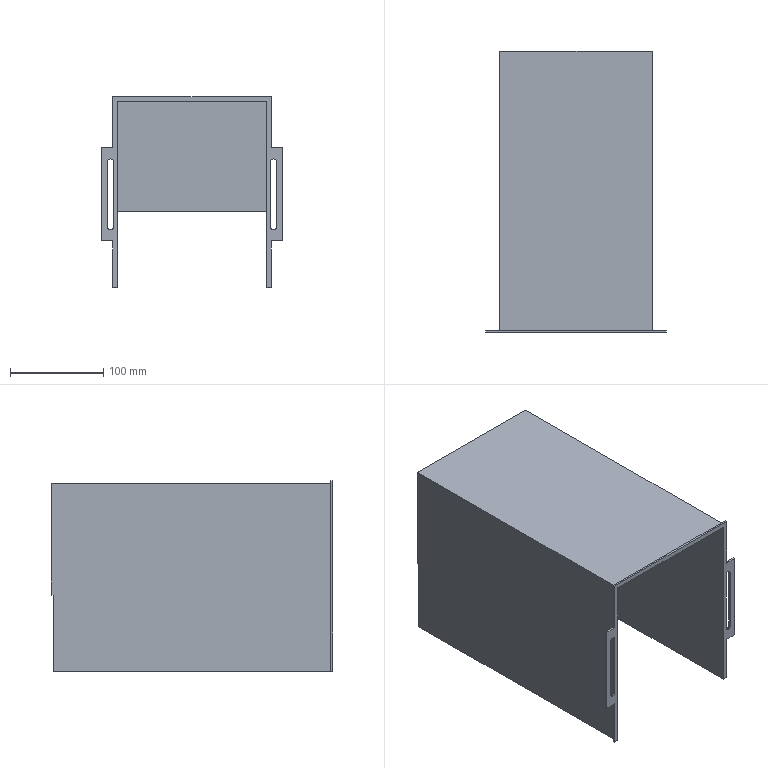Part | SolidWorks | features ICE 4, Extrusion 1 | 1 solid | 36 faces | box 194 x 302 x 205 mm | volume 384147 mm3 | plane 30 | cylinder 6 | commonest cylinder face diameters 6.2 x6
STEP:
#1=CARTESIAN_POINT('',(-4.4,2.,-135.));
#2=VERTEX_POINT('',#1);
#3=CARTESIAN_POINT('',(-7.5,2.,-138.1));
#4=VERTEX_POINT('',#3);
#5=CARTESIAN_POINT('',(-7.5,2.,-135.));
#6=DIRECTION('',(0.,1.,0.));
#7=DIRECTION('',(0.,0.,1.));
#8=AXIS2_PLACEMENT_3D('',#5,#6,#7);
#9=CIRCLE('',#8,3.1);
#10=EDGE_CURVE('',#2,#4,#9,.T.);
#11=ORIENTED_EDGE('',*,*,#10,.T.);
#12=CARTESIAN_POINT('',(-7.5,0.,-138.1));
#13=VERTEX_POINT('',#12);
#14=CARTESIAN_POINT('',(-7.5,300.,-138.1));
#15=DIRECTION('',(0.,-1.,0.));
#16=VECTOR('',#15,1000.);
#17=LINE('',#14,#16);
#18=EDGE_CURVE('',#4,#13,#17,.T.);
#19=ORIENTED_EDGE('',*,*,#18,.T.);
#20=CARTESIAN_POINT('',(-4.4,0.,-135.));
#21=VERTEX_POINT('',#20);
#22=CARTESIAN_POINT('',(-7.5,0.,-135.));
#23=DIRECTION('',(0.,-1.,0.));
#24=DIRECTION('',(0.,0.,-1.));
#25=AXIS2_PLACEMENT_3D('',#22,#23,#24);
#26=CIRCLE('',#25,3.1);
#27=EDGE_CURVE('',#13,#21,#26,.T.);
#28=ORIENTED_EDGE('',*,*,#27,.T.);
#29=CARTESIAN_POINT('',(-4.4,300.,-135.));
#30=DIRECTION('',(0.,-1.,0.));
#31=VECTOR('',#30,1000.);
#32=LINE('',#29,#31);
#33=EDGE_CURVE('',#2,#21,#32,.T.);
#34=ORIENTED_EDGE('',*,*,#33,.F.);
#35=EDGE_LOOP('',(#11,#19,#28,#34));
#36=FACE_OUTER_BOUND('',#35,.T.);
#37=CARTESIAN_POINT('',(-7.5,300.,-135.));
#38=DIRECTION('',(0.,-1.,0.));
#39=DIRECTION('',(0.,0.,-1.));
#40=AXIS2_PLACEMENT_3D('',#37,#38,#39);
#41=CYLINDRICAL_SURFACE('',#40,3.1);
#42=ADVANCED_FACE('',(#36),#41,.F.);
#43=CARTESIAN_POINT('',(167.5,2.,-138.1));
#44=VERTEX_POINT('',#43);
#45=CARTESIAN_POINT('',(170.6,2.,-135.));
#46=VERTEX_POINT('',#45);
#47=CARTESIAN_POINT('',(167.5,2.,-135.));
#48=DIRECTION('',(0.,-1.,0.));
#49=DIRECTION('',(0.,0.,-1.));
#50=AXIS2_PLACEMENT_3D('',#47,#48,#49);
#51=CIRCLE('',#50,3.1);
#52=EDGE_CURVE('',#44,#46,#51,.T.);
#53=ORIENTED_EDGE('',*,*,#52,.F.);
#54=CARTESIAN_POINT('',(167.5,0.,-138.1));
#55=VERTEX_POINT('',#54);
#56=CARTESIAN_POINT('',(167.5,300.,-138.1));
#57=DIRECTION('',(0.,-1.,0.));
#58=VECTOR('',#57,1000.);
#59=LINE('',#56,#58);
#60=EDGE_CURVE('',#44,#55,#59,.T.);
#61=ORIENTED_EDGE('',*,*,#60,.T.);
#62=CARTESIAN_POINT('',(170.6,0.,-135.));
#63=VERTEX_POINT('',#62);
#64=CARTESIAN_POINT('',(167.5,0.,-135.));
#65=DIRECTION('',(0.,-1.,0.));
#66=DIRECTION('',(0.,0.,-1.));
#67=AXIS2_PLACEMENT_3D('',#64,#65,#66);
#68=CIRCLE('',#67,3.1);
#69=EDGE_CURVE('',#55,#63,#68,.T.);
#70=ORIENTED_EDGE('',*,*,#69,.T.);
#71=CARTESIAN_POINT('',(170.6,300.,-135.));
#72=DIRECTION('',(0.,-1.,0.));
#73=VECTOR('',#72,1000.);
#74=LINE('',#71,#73);
#75=EDGE_CURVE('',#46,#63,#74,.T.);
#76=ORIENTED_EDGE('',*,*,#75,.F.);
#77=EDGE_LOOP('',(#53,#61,#70,#76));
#78=FACE_OUTER_BOUND('',#77,.T.);
#79=CARTESIAN_POINT('',(167.5,300.,-135.));
#80=DIRECTION('',(0.,-1.,0.));
#81=DIRECTION('',(0.,0.,-1.));
#82=AXIS2_PLACEMENT_3D('',#79,#80,#81);
#83=CYLINDRICAL_SURFACE('',#82,3.1);
#84=ADVANCED_FACE('',(#78),#83,.F.);
#85=CARTESIAN_POINT('',(162.,2.,2.));
#86=VERTEX_POINT('',#85);
#87=CARTESIAN_POINT('',(162.,2.,-200.));
#88=VERTEX_POINT('',#87);
#89=CARTESIAN_POINT('',(162.,2.,-50.));
#90=DIRECTION('',(0.,0.,-1.));
#91=VECTOR('',#90,1000.);
#92=LINE('',#89,#91);
#93=EDGE_CURVE('',#86,#88,#92,.T.);
#94=ORIENTED_EDGE('',*,*,#93,.T.);
#95=CARTESIAN_POINT('',(162.,300.,-200.));
#96=VERTEX_POINT('',#95);
#97=CARTESIAN_POINT('',(162.,300.,-200.));
#98=DIRECTION('',(0.,-1.,0.));
#99=VECTOR('',#98,1000.);
#100=LINE('',#97,#99);
#101=EDGE_CURVE('',#96,#88,#100,.T.);
#102=ORIENTED_EDGE('',*,*,#101,.F.);
#103=CARTESIAN_POINT('',(162.,300.,-118.));
#104=VERTEX_POINT('',#103);
#105=CARTESIAN_POINT('',(162.,300.,2.));
#106=DIRECTION('',(0.,0.,-1.));
#107=VECTOR('',#106,1000.);
#108=LINE('',#105,#107);
#109=EDGE_CURVE('',#104,#96,#108,.T.);
#110=ORIENTED_EDGE('',*,*,#109,.F.);
#111=CARTESIAN_POINT('',(162.,302.,-118.));
#112=VERTEX_POINT('',#111);
#113=CARTESIAN_POINT('',(162.,302.,-118.));
#114=DIRECTION('',(0.,-1.,0.));
#115=VECTOR('',#114,1000.);
#116=LINE('',#113,#115);
#117=EDGE_CURVE('',#112,#104,#116,.T.);
#118=ORIENTED_EDGE('',*,*,#117,.F.);
#119=CARTESIAN_POINT('',(162.,302.,2.));
#120=VERTEX_POINT('',#119);
#121=CARTESIAN_POINT('',(162.,302.,2.));
#122=DIRECTION('',(0.,0.,-1.));
#123=VECTOR('',#122,1000.);
#124=LINE('',#121,#123);
#125=EDGE_CURVE('',#120,#112,#124,.T.);
#126=ORIENTED_EDGE('',*,*,#125,.F.);
#127=CARTESIAN_POINT('',(162.,300.,2.));
#128=DIRECTION('',(0.,-1.,0.));
#129=VECTOR('',#128,1000.);
#130=LINE('',#127,#129);
#131=EDGE_CURVE('',#120,#86,#130,.T.);
#132=ORIENTED_EDGE('',*,*,#131,.T.);
#133=EDGE_LOOP('',(#94,#102,#110,#118,#126,#132));
#134=FACE_OUTER_BOUND('',#133,.T.);
#135=CARTESIAN_POINT('',(162.,300.,2.));
#136=DIRECTION('',(-1.,0.,0.));
#137=DIRECTION('',(0.,0.,1.));
#138=AXIS2_PLACEMENT_3D('',#135,#136,#137);
#139=PLANE('',#138);
#140=ADVANCED_FACE('',(#134),#139,.F.);
#141=CARTESIAN_POINT('',(-2.,2.,-200.));
#142=VERTEX_POINT('',#141);
#143=CARTESIAN_POINT('',(-2.,2.,2.));
#144=VERTEX_POINT('',#143);
#145=CARTESIAN_POINT('',(-2.,2.,-50.));
#146=DIRECTION('',(0.,0.,1.));
#147=VECTOR('',#146,1000.);
#148=LINE('',#145,#147);
#149=EDGE_CURVE('',#142,#144,#148,.T.);
#150=ORIENTED_EDGE('',*,*,#149,.T.);
#151=CARTESIAN_POINT('',(-2.,302.,2.));
#152=VERTEX_POINT('',#151);
#153=CARTESIAN_POINT('',(-2.,300.,2.));
#154=DIRECTION('',(0.,-1.,0.));
#155=VECTOR('',#154,1000.);
#156=LINE('',#153,#155);
#157=EDGE_CURVE('',#152,#144,#156,.T.);
#158=ORIENTED_EDGE('',*,*,#157,.F.);
#159=CARTESIAN_POINT('',(-2.,302.,-118.));
#160=VERTEX_POINT('',#159);
#161=CARTESIAN_POINT('',(-2.,302.,2.));
#162=DIRECTION('',(0.,0.,1.));
#163=VECTOR('',#162,1000.);
#164=LINE('',#161,#163);
#165=EDGE_CURVE('',#160,#152,#164,.T.);
#166=ORIENTED_EDGE('',*,*,#165,.F.);
#167=CARTESIAN_POINT('',(-2.,300.,-118.));
#168=VERTEX_POINT('',#167);
#169=CARTESIAN_POINT('',(-2.,302.,-118.));
#170=DIRECTION('',(0.,-1.,0.));
#171=VECTOR('',#170,1000.);
#172=LINE('',#169,#171);
#173=EDGE_CURVE('',#160,#168,#172,.T.);
#174=ORIENTED_EDGE('',*,*,#173,.T.);
#175=CARTESIAN_POINT('',(-2.,300.,-200.));
#176=VERTEX_POINT('',#175);
#177=CARTESIAN_POINT('',(-2.,300.,2.));
#178=DIRECTION('',(0.,0.,1.));
#179=VECTOR('',#178,1000.);
#180=LINE('',#177,#179);
#181=EDGE_CURVE('',#176,#168,#180,.T.);
#182=ORIENTED_EDGE('',*,*,#181,.F.);
#183=CARTESIAN_POINT('',(-2.,300.,-200.));
#184=DIRECTION('',(0.,-1.,0.));
#185=VECTOR('',#184,1000.);
#186=LINE('',#183,#185);
#187=EDGE_CURVE('',#176,#142,#186,.T.);
#188=ORIENTED_EDGE('',*,*,#187,.T.);
#189=EDGE_LOOP('',(#150,#158,#166,#174,#182,#188));
#190=FACE_OUTER_BOUND('',#189,.T.);
#191=CARTESIAN_POINT('',(-2.,300.,2.));
#192=DIRECTION('',(1.,0.,0.));
#193=DIRECTION('',(0.,0.,-1.));
#194=AXIS2_PLACEMENT_3D('',#191,#192,#193);
#195=PLANE('',#194);
#196=ADVANCED_FACE('',(#190),#195,.F.);
#197=CARTESIAN_POINT('',(-2.,2.,2.));
#198=DIRECTION('',(1.,0.,0.));
#199=VECTOR('',#198,1000.);
#200=LINE('',#197,#199);
#201=EDGE_CURVE('',#144,#86,#200,.T.);
#202=ORIENTED_EDGE('',*,*,#201,.T.);
#203=ORIENTED_EDGE('',*,*,#131,.F.);
#204=CARTESIAN_POINT('',(-2.,302.,2.));
#205=DIRECTION('',(1.,0.,0.));
#206=VECTOR('',#205,1000.);
#207=LINE('',#204,#206);
#208=EDGE_CURVE('',#152,#120,#207,.T.);
#209=ORIENTED_EDGE('',*,*,#208,.F.);
#210=ORIENTED_EDGE('',*,*,#157,.T.);
#211=EDGE_LOOP('',(#202,#203,#209,#210));
#212=FACE_OUTER_BOUND('',#211,.T.);
#213=CARTESIAN_POINT('',(-2.,300.,2.));
#214=DIRECTION('',(0.,0.,-1.));
#215=DIRECTION('',(-1.,0.,0.));
#216=AXIS2_PLACEMENT_3D('',#213,#214,#215);
#217=PLANE('',#216);
#218=ADVANCED_FACE('',(#212),#217,.F.);
#219=CARTESIAN_POINT('',(160.,300.,-118.));
#220=VERTEX_POINT('',#219);
#221=CARTESIAN_POINT('',(-2.,300.,-118.));
#222=DIRECTION('',(-1.,0.,0.));
#223=VECTOR('',#222,1000.);
#224=LINE('',#221,#223);
#225=EDGE_CURVE('',#104,#220,#224,.T.);
#226=ORIENTED_EDGE('',*,*,#225,.F.);
#227=ORIENTED_EDGE('',*,*,#109,.T.);
#228=CARTESIAN_POINT('',(160.,300.,-200.));
#229=VERTEX_POINT('',#228);
#230=CARTESIAN_POINT('',(160.,300.,-200.));
#231=DIRECTION('',(-1.,0.,0.));
#232=VECTOR('',#231,1000.);
#233=LINE('',#230,#232);
#234=EDGE_CURVE('',#96,#229,#233,.T.);
#235=ORIENTED_EDGE('',*,*,#234,.T.);
#236=CARTESIAN_POINT('',(160.,300.,0.));
#237=DIRECTION('',(0.,0.,1.));
#238=VECTOR('',#237,1000.);
#239=LINE('',#236,#238);
#240=EDGE_CURVE('',#229,#220,#239,.T.);
#241=ORIENTED_EDGE('',*,*,#240,.T.);
#242=EDGE_LOOP('',(#226,#227,#235,#241));
#243=FACE_OUTER_BOUND('',#242,.T.);
#244=CARTESIAN_POINT('',(0.,300.,0.));
#245=DIRECTION('',(0.,1.,0.));
#246=DIRECTION('',(0.,0.,1.));
#247=AXIS2_PLACEMENT_3D('',#244,#245,#246);
#248=PLANE('',#247);
#249=ADVANCED_FACE('',(#243),#248,.T.);
#250=CARTESIAN_POINT('',(160.,0.,0.));
#251=VERTEX_POINT('',#250);
#252=CARTESIAN_POINT('',(0.,0.,0.));
#253=VERTEX_POINT('',#252);
#254=CARTESIAN_POINT('',(0.,0.,0.));
#255=DIRECTION('',(-1.,0.,0.));
#256=VECTOR('',#255,1000.);
#257=LINE('',#254,#256);
#258=EDGE_CURVE('',#251,#253,#257,.T.);
#259=ORIENTED_EDGE('',*,*,#258,.T.);
#260=CARTESIAN_POINT('',(0.,300.,0.));
#261=VERTEX_POINT('',#260);
#262=CARTESIAN_POINT('',(0.,300.,0.));
#263=DIRECTION('',(0.,-1.,0.));
#264=VECTOR('',#263,1000.);
#265=LINE('',#262,#264);
#266=EDGE_CURVE('',#261,#253,#265,.T.);
#267=ORIENTED_EDGE('',*,*,#266,.F.);
#268=CARTESIAN_POINT('',(160.,300.,0.));
#269=VERTEX_POINT('',#268);
#270=CARTESIAN_POINT('',(0.,300.,0.));
#271=DIRECTION('',(-1.,0.,0.));
#272=VECTOR('',#271,1000.);
#273=LINE('',#270,#272);
#274=EDGE_CURVE('',#269,#261,#273,.T.);
#275=ORIENTED_EDGE('',*,*,#274,.F.);
#276=CARTESIAN_POINT('',(160.,300.,0.));
#277=DIRECTION('',(0.,-1.,0.));
#278=VECTOR('',#277,1000.);
#279=LINE('',#276,#278);
#280=EDGE_CURVE('',#269,#251,#279,.T.);
#281=ORIENTED_EDGE('',*,*,#280,.T.);
#282=EDGE_LOOP('',(#259,#267,#275,#281));
#283=FACE_OUTER_BOUND('',#282,.T.);
#284=CARTESIAN_POINT('',(0.,300.,0.));
#285=DIRECTION('',(0.,0.,1.));
#286=DIRECTION('',(1.,0.,0.));
#287=AXIS2_PLACEMENT_3D('',#284,#285,#286);
#288=PLANE('',#287);
#289=ADVANCED_FACE('',(#283),#288,.F.);
#290=CARTESIAN_POINT('',(0.,0.,-200.));
#291=VERTEX_POINT('',#290);
#292=CARTESIAN_POINT('',(0.,0.,0.));
#293=DIRECTION('',(0.,0.,-1.));
#294=VECTOR('',#293,1000.);
#295=LINE('',#292,#294);
#296=EDGE_CURVE('',#253,#291,#295,.T.);
#297=ORIENTED_EDGE('',*,*,#296,.T.);
#298=CARTESIAN_POINT('',(0.,300.,-200.));
#299=VERTEX_POINT('',#298);
#300=CARTESIAN_POINT('',(0.,300.,-200.));
#301=DIRECTION('',(0.,-1.,0.));
#302=VECTOR('',#301,1000.);
#303=LINE('',#300,#302);
#304=EDGE_CURVE('',#299,#291,#303,.T.);
#305=ORIENTED_EDGE('',*,*,#304,.F.);
#306=CARTESIAN_POINT('',(0.,300.,-118.));
#307=VERTEX_POINT('',#306);
#308=CARTESIAN_POINT('',(0.,300.,0.));
#309=DIRECTION('',(0.,0.,-1.));
#310=VECTOR('',#309,1000.);
#311=LINE('',#308,#310);
#312=EDGE_CURVE('',#307,#299,#311,.T.);
#313=ORIENTED_EDGE('',*,*,#312,.F.);
#314=CARTESIAN_POINT('',(0.,300.,0.));
#315=DIRECTION('',(0.,0.,-1.));
#316=VECTOR('',#315,1000.);
#317=LINE('',#314,#316);
#318=EDGE_CURVE('',#261,#307,#317,.T.);
#319=ORIENTED_EDGE('',*,*,#318,.F.);
#320=ORIENTED_EDGE('',*,*,#266,.T.);
#321=EDGE_LOOP('',(#297,#305,#313,#319,#320));
#322=FACE_OUTER_BOUND('',#321,.T.);
#323=CARTESIAN_POINT('',(0.,300.,0.));
#324=DIRECTION('',(-1.,0.,0.));
#325=DIRECTION('',(0.,0.,1.));
#326=AXIS2_PLACEMENT_3D('',#323,#324,#325);
#327=PLANE('',#326);
#328=ADVANCED_FACE('',(#322),#327,.F.);
#329=CARTESIAN_POINT('',(-5.,0.,-200.));
#330=VERTEX_POINT('',#329);
#331=CARTESIAN_POINT('',(-2.,0.,-200.));
#332=DIRECTION('',(-1.,0.,0.));
#333=VECTOR('',#332,1000.);
#334=LINE('',#331,#333);
#335=EDGE_CURVE('',#291,#330,#334,.T.);
#336=ORIENTED_EDGE('',*,*,#335,.T.);
#337=CARTESIAN_POINT('',(-5.,2.,-200.));
#338=VERTEX_POINT('',#337);
#339=CARTESIAN_POINT('',(-5.,2.,-200.));
#340=DIRECTION('',(0.,-1.,0.));
#341=VECTOR('',#340,1000.);
#342=LINE('',#339,#341);
#343=EDGE_CURVE('',#338,#330,#342,.T.);
#344=ORIENTED_EDGE('',*,*,#343,.F.);
#345=CARTESIAN_POINT('',(-5.,2.,-200.));
#346=DIRECTION('',(1.,0.,0.));
#347=VECTOR('',#346,1000.);
#348=LINE('',#345,#347);
#349=EDGE_CURVE('',#338,#142,#348,.T.);
#350=ORIENTED_EDGE('',*,*,#349,.T.);
#351=ORIENTED_EDGE('',*,*,#187,.F.);
#352=CARTESIAN_POINT('',(-2.,300.,-200.));
#353=DIRECTION('',(-1.,0.,0.));
#354=VECTOR('',#353,1000.);
#355=LINE('',#352,#354);
#356=EDGE_CURVE('',#299,#176,#355,.T.);
#357=ORIENTED_EDGE('',*,*,#356,.F.);
#358=ORIENTED_EDGE('',*,*,#304,.T.);
#359=EDGE_LOOP('',(#336,#344,#350,#351,#357,#358));
#360=FACE_OUTER_BOUND('',#359,.T.);
#361=CARTESIAN_POINT('',(-2.,300.,-200.));
#362=DIRECTION('',(0.,0.,1.));
#363=DIRECTION('',(1.,0.,0.));
#364=AXIS2_PLACEMENT_3D('',#361,#362,#363);
#365=PLANE('',#364);
#366=ADVANCED_FACE('',(#360),#365,.F.);
#367=CARTESIAN_POINT('',(165.,0.,-200.));
#368=VERTEX_POINT('',#367);
#369=CARTESIAN_POINT('',(160.,0.,-200.));
#370=VERTEX_POINT('',#369);
#371=CARTESIAN_POINT('',(160.,0.,-200.));
#372=DIRECTION('',(-1.,0.,0.));
#373=VECTOR('',#372,1000.);
#374=LINE('',#371,#373);
#375=EDGE_CURVE('',#368,#370,#374,.T.);
#376=ORIENTED_EDGE('',*,*,#375,.T.);
#377=CARTESIAN_POINT('',(160.,300.,-200.));
#378=DIRECTION('',(0.,-1.,0.));
#379=VECTOR('',#378,1000.);
#380=LINE('',#377,#379);
#381=EDGE_CURVE('',#229,#370,#380,.T.);
#382=ORIENTED_EDGE('',*,*,#381,.F.);
#383=ORIENTED_EDGE('',*,*,#234,.F.);
#384=ORIENTED_EDGE('',*,*,#101,.T.);
#385=CARTESIAN_POINT('',(165.,2.,-200.));
#386=VERTEX_POINT('',#385);
#387=CARTESIAN_POINT('',(162.,2.,-200.));
#388=DIRECTION('',(1.,0.,0.));
#389=VECTOR('',#388,1000.);
#390=LINE('',#387,#389);
#391=EDGE_CURVE('',#88,#386,#390,.T.);
#392=ORIENTED_EDGE('',*,*,#391,.T.);
#393=CARTESIAN_POINT('',(165.,2.,-200.));
#394=DIRECTION('',(0.,-1.,0.));
#395=VECTOR('',#394,1000.);
#396=LINE('',#393,#395);
#397=EDGE_CURVE('',#386,#368,#396,.T.);
#398=ORIENTED_EDGE('',*,*,#397,.T.);
#399=EDGE_LOOP('',(#376,#382,#383,#384,#392,#398));
#400=FACE_OUTER_BOUND('',#399,.T.);
#401=CARTESIAN_POINT('',(160.,300.,-200.));
#402=DIRECTION('',(0.,0.,1.));
#403=DIRECTION('',(1.,0.,0.));
#404=AXIS2_PLACEMENT_3D('',#401,#402,#403);
#405=PLANE('',#404);
#406=ADVANCED_FACE('',(#400),#405,.F.);
#407=CARTESIAN_POINT('',(160.,0.,0.));
#408=DIRECTION('',(0.,0.,1.));
#409=VECTOR('',#408,1000.);
#410=LINE('',#407,#409);
#411=EDGE_CURVE('',#370,#251,#410,.T.);
#412=ORIENTED_EDGE('',*,*,#411,.T.);
#413=ORIENTED_EDGE('',*,*,#280,.F.);
#414=CARTESIAN_POINT('',(160.,300.,0.));
#415=DIRECTION('',(0.,0.,1.));
#416=VECTOR('',#415,1000.);
#417=LINE('',#414,#416);
#418=EDGE_CURVE('',#220,#269,#417,.T.);
#419=ORIENTED_EDGE('',*,*,#418,.F.);
#420=ORIENTED_EDGE('',*,*,#240,.F.);
#421=ORIENTED_EDGE('',*,*,#381,.T.);
#422=EDGE_LOOP('',(#412,#413,#419,#420,#421));
#423=FACE_OUTER_BOUND('',#422,.T.);
#424=CARTESIAN_POINT('',(160.,300.,0.));
#425=DIRECTION('',(1.,0.,0.));
#426=DIRECTION('',(0.,0.,-1.));
#427=AXIS2_PLACEMENT_3D('',#424,#425,#426);
#428=PLANE('',#427);
#429=ADVANCED_FACE('',(#423),#428,.F.);
#430=CARTESIAN_POINT('',(-2.,300.,-118.));
#431=DIRECTION('',(-1.,0.,0.));
#432=VECTOR('',#431,1000.);
#433=LINE('',#430,#432);
#434=EDGE_CURVE('',#307,#168,#433,.T.);
#435=ORIENTED_EDGE('',*,*,#434,.F.);
#436=ORIENTED_EDGE('',*,*,#312,.T.);
#437=ORIENTED_EDGE('',*,*,#356,.T.);
#438=ORIENTED_EDGE('',*,*,#181,.T.);
#439=EDGE_LOOP('',(#435,#436,#437,#438));
#440=FACE_OUTER_BOUND('',#439,.T.);
#441=CARTESIAN_POINT('',(0.,300.,0.));
#442=DIRECTION('',(0.,1.,0.));
#443=DIRECTION('',(0.,0.,1.));
#444=AXIS2_PLACEMENT_3D('',#441,#442,#443);
#445=PLANE('',#444);
#446=ADVANCED_FACE('',(#440),#445,.T.);
#447=ORIENTED_EDGE('',*,*,#375,.F.);
#448=CARTESIAN_POINT('',(165.,0.,-150.));
#449=VERTEX_POINT('',#448);
#450=CARTESIAN_POINT('',(165.,0.,-137.967));
#451=DIRECTION('',(0.,0.,1.));
#452=VECTOR('',#451,1000.);
#453=LINE('',#450,#452);
#454=EDGE_CURVE('',#368,#449,#453,.T.);
#455=ORIENTED_EDGE('',*,*,#454,.T.);
#456=CARTESIAN_POINT('',(177.,0.,-150.));
#457=VERTEX_POINT('',#456);
#458=CARTESIAN_POINT('',(162.,0.,-150.));
#459=DIRECTION('',(1.,0.,0.));
#460=VECTOR('',#459,1000.);
#461=LINE('',#458,#460);
#462=EDGE_CURVE('',#449,#457,#461,.T.);
#463=ORIENTED_EDGE('',*,*,#462,.T.);
#464=CARTESIAN_POINT('',(177.,0.,-50.));
#465=VERTEX_POINT('',#464);
#466=CARTESIAN_POINT('',(177.,0.,-50.));
#467=DIRECTION('',(0.,0.,1.));
#468=VECTOR('',#467,1000.);
#469=LINE('',#466,#468);
#470=EDGE_CURVE('',#457,#465,#469,.T.);
#471=ORIENTED_EDGE('',*,*,#470,.T.);
#472=CARTESIAN_POINT('',(165.,0.,-50.));
#473=VERTEX_POINT('',#472);
#474=CARTESIAN_POINT('',(162.,0.,-50.));
#475=DIRECTION('',(-1.,0.,0.));
#476=VECTOR('',#475,1000.);
#477=LINE('',#474,#476);
#478=EDGE_CURVE('',#465,#473,#477,.T.);
#479=ORIENTED_EDGE('',*,*,#478,.T.);
#480=CARTESIAN_POINT('',(165.,0.,5.));
#481=VERTEX_POINT('',#480);
#482=CARTESIAN_POINT('',(165.,0.,5.));
#483=DIRECTION('',(0.,0.,1.));
#484=VECTOR('',#483,1000.);
#485=LINE('',#482,#484);
#486=EDGE_CURVE('',#473,#481,#485,.T.);
#487=ORIENTED_EDGE('',*,*,#486,.T.);
#488=CARTESIAN_POINT('',(-5.,0.,5.));
#489=VERTEX_POINT('',#488);
#490=CARTESIAN_POINT('',(-5.,0.,5.));
#491=DIRECTION('',(-1.,0.,0.));
#492=VECTOR('',#491,1000.);
#493=LINE('',#490,#492);
#494=EDGE_CURVE('',#481,#489,#493,.T.);
#495=ORIENTED_EDGE('',*,*,#494,.T.);
#496=CARTESIAN_POINT('',(-5.,0.,-50.));
#497=VERTEX_POINT('',#496);
#498=CARTESIAN_POINT('',(-5.,0.,-59.254));
#499=DIRECTION('',(0.,0.,-1.));
#500=VECTOR('',#499,1000.);
#501=LINE('',#498,#500);
#502=EDGE_CURVE('',#489,#497,#501,.T.);
#503=ORIENTED_EDGE('',*,*,#502,.T.);
#504=CARTESIAN_POINT('',(-17.,0.,-50.));
#505=VERTEX_POINT('',#504);
#506=CARTESIAN_POINT('',(-2.,0.,-50.));
#507=DIRECTION('',(-1.,0.,0.));
#508=VECTOR('',#507,1000.);
#509=LINE('',#506,#508);
#510=EDGE_CURVE('',#497,#505,#509,.T.);
#511=ORIENTED_EDGE('',*,*,#510,.T.);
#512=CARTESIAN_POINT('',(-17.,0.,-150.));
#513=VERTEX_POINT('',#512);
#514=CARTESIAN_POINT('',(-17.,0.,-50.));
#515=DIRECTION('',(0.,0.,-1.));
#516=VECTOR('',#515,1000.);
#517=LINE('',#514,#516);
#518=EDGE_CURVE('',#505,#513,#517,.T.);
#519=ORIENTED_EDGE('',*,*,#518,.T.);
#520=CARTESIAN_POINT('',(-5.,0.,-150.));
#521=VERTEX_POINT('',#520);
#522=CARTESIAN_POINT('',(-2.,0.,-150.));
#523=DIRECTION('',(1.,0.,0.));
#524=VECTOR('',#523,1000.);
#525=LINE('',#522,#524);
#526=EDGE_CURVE('',#513,#521,#525,.T.);
#527=ORIENTED_EDGE('',*,*,#526,.T.);
#528=CARTESIAN_POINT('',(-5.,0.,-200.));
#529=DIRECTION('',(0.,0.,-1.));
#530=VECTOR('',#529,1000.);
#531=LINE('',#528,#530);
#532=EDGE_CURVE('',#521,#330,#531,.T.);
#533=ORIENTED_EDGE('',*,*,#532,.T.);
#534=ORIENTED_EDGE('',*,*,#335,.F.);
#535=ORIENTED_EDGE('',*,*,#296,.F.);
#536=ORIENTED_EDGE('',*,*,#258,.F.);
#537=ORIENTED_EDGE('',*,*,#411,.F.);
#538=EDGE_LOOP('',(#447,#455,#463,#471,#479,#487,#495,#503,#511,#519,#527,#533,#534,#535,#536,#537));
#539=FACE_OUTER_BOUND('',#538,.T.);
#540=CARTESIAN_POINT('',(164.4,0.,-65.));
#541=VERTEX_POINT('',#540);
#542=CARTESIAN_POINT('',(164.4,0.,-135.));
#543=VERTEX_POINT('',#542);
#544=CARTESIAN_POINT('',(164.4,0.,-65.));
#545=DIRECTION('',(0.,0.,-1.));
#546=VECTOR('',#545,1000.);
#547=LINE('',#544,#546);
#548=EDGE_CURVE('',#541,#543,#547,.T.);
#549=ORIENTED_EDGE('',*,*,#548,.F.);
#550=CARTESIAN_POINT('',(170.6,0.,-65.));
#551=VERTEX_POINT('',#550);
#552=CARTESIAN_POINT('',(167.5,0.,-65.));
#553=DIRECTION('',(0.,-1.,0.));
#554=DIRECTION('',(0.,0.,-1.));
#555=AXIS2_PLACEMENT_3D('',#552,#553,#554);
#556=CIRCLE('',#555,3.1);
#557=EDGE_CURVE('',#551,#541,#556,.T.);
#558=ORIENTED_EDGE('',*,*,#557,.F.);
#559=CARTESIAN_POINT('',(170.6,0.,-65.));
#560=DIRECTION('',(0.,0.,1.));
#561=VECTOR('',#560,1000.);
#562=LINE('',#559,#561);
#563=EDGE_CURVE('',#63,#551,#562,.T.);
#564=ORIENTED_EDGE('',*,*,#563,.F.);
#565=ORIENTED_EDGE('',*,*,#69,.F.);
#566=CARTESIAN_POINT('',(167.5,0.,-135.));
#567=DIRECTION('',(0.,-1.,0.));
#568=DIRECTION('',(0.,0.,-1.));
#569=AXIS2_PLACEMENT_3D('',#566,#567,#568);
#570=CIRCLE('',#569,3.1);
#571=EDGE_CURVE('',#543,#55,#570,.T.);
#572=ORIENTED_EDGE('',*,*,#571,.F.);
#573=EDGE_LOOP('',(#549,#558,#564,#565,#572));
#574=FACE_BOUND('',#573,.T.);
#575=CARTESIAN_POINT('',(-10.6,0.,-65.));
#576=VERTEX_POINT('',#575);
#577=CARTESIAN_POINT('',(-10.6,0.,-135.));
#578=VERTEX_POINT('',#577);
#579=CARTESIAN_POINT('',(-10.6,0.,-65.));
#580=DIRECTION('',(0.,0.,-1.));
#581=VECTOR('',#580,1000.);
#582=LINE('',#579,#581);
#583=EDGE_CURVE('',#576,#578,#582,.T.);
#584=ORIENTED_EDGE('',*,*,#583,.F.);
#585=CARTESIAN_POINT('',(-4.4,0.,-65.));
#586=VERTEX_POINT('',#585);
#587=CARTESIAN_POINT('',(-7.5,0.,-65.));
#588=DIRECTION('',(0.,-1.,0.));
#589=DIRECTION('',(0.,0.,-1.));
#590=AXIS2_PLACEMENT_3D('',#587,#588,#589);
#591=CIRCLE('',#590,3.1);
#592=EDGE_CURVE('',#586,#576,#591,.T.);
#593=ORIENTED_EDGE('',*,*,#592,.F.);
#594=CARTESIAN_POINT('',(-4.4,0.,-65.));
#595=DIRECTION('',(0.,0.,1.));
#596=VECTOR('',#595,1000.);
#597=LINE('',#594,#596);
#598=EDGE_CURVE('',#21,#586,#597,.T.);
#599=ORIENTED_EDGE('',*,*,#598,.F.);
#600=ORIENTED_EDGE('',*,*,#27,.F.);
#601=CARTESIAN_POINT('',(-7.5,0.,-135.));
#602=DIRECTION('',(0.,-1.,0.));
#603=DIRECTION('',(0.,0.,-1.));
#604=AXIS2_PLACEMENT_3D('',#601,#602,#603);
#605=CIRCLE('',#604,3.1);
#606=EDGE_CURVE('',#578,#13,#605,.T.);
#607=ORIENTED_EDGE('',*,*,#606,.F.);
#608=EDGE_LOOP('',(#584,#593,#599,#600,#607));
#609=FACE_BOUND('',#608,.T.);
#610=CARTESIAN_POINT('',(0.,0.,0.));
#611=DIRECTION('',(0.,1.,0.));
#612=DIRECTION('',(0.,0.,1.));
#613=AXIS2_PLACEMENT_3D('',#610,#611,#612);
#614=PLANE('',#613);
#615=ADVANCED_FACE('',(#539,#574,#609),#614,.F.);
#616=CARTESIAN_POINT('',(-5.,2.,-150.));
#617=VERTEX_POINT('',#616);
#618=CARTESIAN_POINT('',(-5.,2.,-150.));
#619=DIRECTION('',(0.,1.,0.));
#620=VECTOR('',#619,1000.);
#621=LINE('',#618,#620);
#622=EDGE_CURVE('',#521,#617,#621,.T.);
#623=ORIENTED_EDGE('',*,*,#622,.F.);
#624=ORIENTED_EDGE('',*,*,#526,.F.);
#625=CARTESIAN_POINT('',(-17.,2.,-150.));
#626=VERTEX_POINT('',#625);
#627=CARTESIAN_POINT('',(-17.,2.,-150.));
#628=DIRECTION('',(0.,-1.,0.));
#629=VECTOR('',#628,1000.);
#630=LINE('',#627,#629);
#631=EDGE_CURVE('',#626,#513,#630,.T.);
#632=ORIENTED_EDGE('',*,*,#631,.F.);
#633=CARTESIAN_POINT('',(-2.,2.,-150.));
#634=DIRECTION('',(1.,0.,0.));
#635=VECTOR('',#634,1000.);
#636=LINE('',#633,#635);
#637=EDGE_CURVE('',#626,#617,#636,.T.);
#638=ORIENTED_EDGE('',*,*,#637,.T.);
#639=EDGE_LOOP('',(#623,#624,#632,#638));
#640=FACE_OUTER_BOUND('',#639,.T.);
#641=CARTESIAN_POINT('',(-2.,2.,-150.));
#642=DIRECTION('',(0.,0.,-1.));
#643=DIRECTION('',(-1.,0.,0.));
#644=AXIS2_PLACEMENT_3D('',#641,#642,#643);
#645=PLANE('',#644);
#646=ADVANCED_FACE('',(#640),#645,.T.);
#647=ORIENTED_EDGE('',*,*,#518,.F.);
#648=CARTESIAN_POINT('',(-17.,2.,-50.));
#649=VERTEX_POINT('',#648);
#650=CARTESIAN_POINT('',(-17.,2.,-50.));
#651=DIRECTION('',(0.,-1.,0.));
#652=VECTOR('',#651,1000.);
#653=LINE('',#650,#652);
#654=EDGE_CURVE('',#649,#505,#653,.T.);
#655=ORIENTED_EDGE('',*,*,#654,.F.);
#656=CARTESIAN_POINT('',(-17.,2.,-50.));
#657=DIRECTION('',(0.,0.,-1.));
#658=VECTOR('',#657,1000.);
#659=LINE('',#656,#658);
#660=EDGE_CURVE('',#649,#626,#659,.T.);
#661=ORIENTED_EDGE('',*,*,#660,.T.);
#662=ORIENTED_EDGE('',*,*,#631,.T.);
#663=EDGE_LOOP('',(#647,#655,#661,#662));
#664=FACE_OUTER_BOUND('',#663,.T.);
#665=CARTESIAN_POINT('',(-17.,2.,-50.));
#666=DIRECTION('',(-1.,0.,0.));
#667=DIRECTION('',(0.,0.,1.));
#668=AXIS2_PLACEMENT_3D('',#665,#666,#667);
#669=PLANE('',#668);
#670=ADVANCED_FACE('',(#664),#669,.T.);
#671=CARTESIAN_POINT('',(-5.,2.,-50.));
#672=VERTEX_POINT('',#671);
#673=CARTESIAN_POINT('',(-5.,2.,-50.));
#674=DIRECTION('',(0.,-1.,0.));
#675=VECTOR('',#674,1000.);
#676=LINE('',#673,#675);
#677=EDGE_CURVE('',#672,#497,#676,.T.);
#678=ORIENTED_EDGE('',*,*,#677,.F.);
#679=CARTESIAN_POINT('',(-2.,2.,-50.));
#680=DIRECTION('',(-1.,0.,0.));
#681=VECTOR('',#680,1000.);
#682=LINE('',#679,#681);
#683=EDGE_CURVE('',#672,#649,#682,.T.);
#684=ORIENTED_EDGE('',*,*,#683,.T.);
#685=ORIENTED_EDGE('',*,*,#654,.T.);
#686=ORIENTED_EDGE('',*,*,#510,.F.);
#687=EDGE_LOOP('',(#678,#684,#685,#686));
#688=FACE_OUTER_BOUND('',#687,.T.);
#689=CARTESIAN_POINT('',(-2.,2.,-50.));
#690=DIRECTION('',(0.,0.,1.));
#691=DIRECTION('',(1.,0.,0.));
#692=AXIS2_PLACEMENT_3D('',#689,#690,#691);
#693=PLANE('',#692);
#694=ADVANCED_FACE('',(#688),#693,.T.);
#695=ORIENTED_EDGE('',*,*,#149,.F.);
#696=ORIENTED_EDGE('',*,*,#349,.F.);
#697=CARTESIAN_POINT('',(-5.,2.,-200.));
#698=DIRECTION('',(0.,0.,-1.));
#699=VECTOR('',#698,1000.);
#700=LINE('',#697,#699);
#701=EDGE_CURVE('',#617,#338,#700,.T.);
#702=ORIENTED_EDGE('',*,*,#701,.F.);
#703=ORIENTED_EDGE('',*,*,#637,.F.);
#704=ORIENTED_EDGE('',*,*,#660,.F.);
#705=ORIENTED_EDGE('',*,*,#683,.F.);
#706=CARTESIAN_POINT('',(-5.,2.,5.));
#707=VERTEX_POINT('',#706);
#708=CARTESIAN_POINT('',(-5.,2.,-59.254));
#709=DIRECTION('',(0.,0.,-1.));
#710=VECTOR('',#709,1000.);
#711=LINE('',#708,#710);
#712=EDGE_CURVE('',#707,#672,#711,.T.);
#713=ORIENTED_EDGE('',*,*,#712,.F.);
#714=CARTESIAN_POINT('',(165.,2.,5.));
#715=VERTEX_POINT('',#714);
#716=CARTESIAN_POINT('',(-5.,2.,5.));
#717=DIRECTION('',(-1.,0.,0.));
#718=VECTOR('',#717,1000.);
#719=LINE('',#716,#718);
#720=EDGE_CURVE('',#715,#707,#719,.T.);
#721=ORIENTED_EDGE('',*,*,#720,.F.);
#722=CARTESIAN_POINT('',(165.,2.,-50.));
#723=VERTEX_POINT('',#722);
#724=CARTESIAN_POINT('',(165.,2.,5.));
#725=DIRECTION('',(0.,0.,1.));
#726=VECTOR('',#725,1000.);
#727=LINE('',#724,#726);
#728=EDGE_CURVE('',#723,#715,#727,.T.);
#729=ORIENTED_EDGE('',*,*,#728,.F.);
#730=CARTESIAN_POINT('',(177.,2.,-50.));
#731=VERTEX_POINT('',#730);
#732=CARTESIAN_POINT('',(162.,2.,-50.));
#733=DIRECTION('',(-1.,0.,0.));
#734=VECTOR('',#733,1000.);
#735=LINE('',#732,#734);
#736=EDGE_CURVE('',#731,#723,#735,.T.);
#737=ORIENTED_EDGE('',*,*,#736,.F.);
#738=CARTESIAN_POINT('',(177.,2.,-150.));
#739=VERTEX_POINT('',#738);
#740=CARTESIAN_POINT('',(177.,2.,-50.));
#741=DIRECTION('',(0.,0.,1.));
#742=VECTOR('',#741,1000.);
#743=LINE('',#740,#742);
#744=EDGE_CURVE('',#739,#731,#743,.T.);
#745=ORIENTED_EDGE('',*,*,#744,.F.);
#746=CARTESIAN_POINT('',(165.,2.,-150.));
#747=VERTEX_POINT('',#746);
#748=CARTESIAN_POINT('',(162.,2.,-150.));
#749=DIRECTION('',(1.,0.,0.));
#750=VECTOR('',#749,1000.);
#751=LINE('',#748,#750);
#752=EDGE_CURVE('',#747,#739,#751,.T.);
#753=ORIENTED_EDGE('',*,*,#752,.F.);
#754=CARTESIAN_POINT('',(165.,2.,-137.967));
#755=DIRECTION('',(0.,0.,1.));
#756=VECTOR('',#755,1000.);
#757=LINE('',#754,#756);
#758=EDGE_CURVE('',#386,#747,#757,.T.);
#759=ORIENTED_EDGE('',*,*,#758,.F.);
#760=ORIENTED_EDGE('',*,*,#391,.F.);
#761=ORIENTED_EDGE('',*,*,#93,.F.);
#762=ORIENTED_EDGE('',*,*,#201,.F.);
#763=EDGE_LOOP('',(#695,#696,#702,#703,#704,#705,#713,#721,#729,#737,#745,#753,#759,#760,#761,#762));
#764=FACE_OUTER_BOUND('',#763,.T.);
#765=CARTESIAN_POINT('',(-10.6,2.,-65.));
#766=VERTEX_POINT('',#765);
#767=CARTESIAN_POINT('',(-4.4,2.,-65.));
#768=VERTEX_POINT('',#767);
#769=CARTESIAN_POINT('',(-7.5,2.,-65.));
#770=DIRECTION('',(0.,1.,0.));
#771=DIRECTION('',(0.,0.,1.));
#772=AXIS2_PLACEMENT_3D('',#769,#770,#771);
#773=CIRCLE('',#772,3.1);
#774=EDGE_CURVE('',#766,#768,#773,.T.);
#775=ORIENTED_EDGE('',*,*,#774,.F.);
#776=CARTESIAN_POINT('',(-10.6,2.,-135.));
#777=VERTEX_POINT('',#776);
#778=CARTESIAN_POINT('',(-10.6,2.,0.));
#779=DIRECTION('',(0.,0.,1.));
#780=VECTOR('',#779,1000.);
#781=LINE('',#778,#780);
#782=EDGE_CURVE('',#777,#766,#781,.T.);
#783=ORIENTED_EDGE('',*,*,#782,.F.);
#784=CARTESIAN_POINT('',(-7.5,2.,-135.));
#785=DIRECTION('',(0.,1.,0.));
#786=DIRECTION('',(0.,0.,1.));
#787=AXIS2_PLACEMENT_3D('',#784,#785,#786);
#788=CIRCLE('',#787,3.1);
#789=EDGE_CURVE('',#4,#777,#788,.T.);
#790=ORIENTED_EDGE('',*,*,#789,.F.);
#791=ORIENTED_EDGE('',*,*,#10,.F.);
#792=CARTESIAN_POINT('',(-4.4,2.,0.));
#793=DIRECTION('',(0.,0.,-1.));
#794=VECTOR('',#793,1000.);
#795=LINE('',#792,#794);
#796=EDGE_CURVE('',#768,#2,#795,.T.);
#797=ORIENTED_EDGE('',*,*,#796,.F.);
#798=EDGE_LOOP('',(#775,#783,#790,#791,#797));
#799=FACE_BOUND('',#798,.T.);
#800=CARTESIAN_POINT('',(170.6,2.,-65.));
#801=VERTEX_POINT('',#800);
#802=CARTESIAN_POINT('',(170.6,2.,0.));
#803=DIRECTION('',(0.,0.,1.));
#804=VECTOR('',#803,1000.);
#805=LINE('',#802,#804);
#806=EDGE_CURVE('',#46,#801,#805,.T.);
#807=ORIENTED_EDGE('',*,*,#806,.T.);
#808=CARTESIAN_POINT('',(164.4,2.,-65.));
#809=VERTEX_POINT('',#808);
#810=CARTESIAN_POINT('',(167.5,2.,-65.));
#811=DIRECTION('',(0.,-1.,0.));
#812=DIRECTION('',(0.,0.,-1.));
#813=AXIS2_PLACEMENT_3D('',#810,#811,#812);
#814=CIRCLE('',#813,3.1);
#815=EDGE_CURVE('',#801,#809,#814,.T.);
#816=ORIENTED_EDGE('',*,*,#815,.T.);
#817=CARTESIAN_POINT('',(164.4,2.,-135.));
#818=VERTEX_POINT('',#817);
#819=CARTESIAN_POINT('',(164.4,2.,0.));
#820=DIRECTION('',(0.,0.,-1.));
#821=VECTOR('',#820,1000.);
#822=LINE('',#819,#821);
#823=EDGE_CURVE('',#809,#818,#822,.T.);
#824=ORIENTED_EDGE('',*,*,#823,.T.);
#825=CARTESIAN_POINT('',(167.5,2.,-135.));
#826=DIRECTION('',(0.,-1.,0.));
#827=DIRECTION('',(0.,0.,-1.));
#828=AXIS2_PLACEMENT_3D('',#825,#826,#827);
#829=CIRCLE('',#828,3.1);
#830=EDGE_CURVE('',#818,#44,#829,.T.);
#831=ORIENTED_EDGE('',*,*,#830,.T.);
#832=ORIENTED_EDGE('',*,*,#52,.T.);
#833=EDGE_LOOP('',(#807,#816,#824,#831,#832));
#834=FACE_BOUND('',#833,.T.);
#835=CARTESIAN_POINT('',(0.,2.,0.));
#836=DIRECTION('',(0.,1.,0.));
#837=DIRECTION('',(0.,0.,1.));
#838=AXIS2_PLACEMENT_3D('',#835,#836,#837);
#839=PLANE('',#838);
#840=ADVANCED_FACE('',(#764,#799,#834),#839,.T.);
#841=CARTESIAN_POINT('',(165.,2.,-50.));
#842=DIRECTION('',(0.,1.,0.));
#843=VECTOR('',#842,1000.);
#844=LINE('',#841,#843);
#845=EDGE_CURVE('',#473,#723,#844,.T.);
#846=ORIENTED_EDGE('',*,*,#845,.F.);
#847=ORIENTED_EDGE('',*,*,#478,.F.);
#848=CARTESIAN_POINT('',(177.,2.,-50.));
#849=DIRECTION('',(0.,-1.,0.));
#850=VECTOR('',#849,1000.);
#851=LINE('',#848,#850);
#852=EDGE_CURVE('',#731,#465,#851,.T.);
#853=ORIENTED_EDGE('',*,*,#852,.F.);
#854=ORIENTED_EDGE('',*,*,#736,.T.);
#855=EDGE_LOOP('',(#846,#847,#853,#854));
#856=FACE_OUTER_BOUND('',#855,.T.);
#857=CARTESIAN_POINT('',(162.,2.,-50.));
#858=DIRECTION('',(0.,0.,1.));
#859=DIRECTION('',(1.,0.,0.));
#860=AXIS2_PLACEMENT_3D('',#857,#858,#859);
#861=PLANE('',#860);
#862=ADVANCED_FACE('',(#856),#861,.T.);
#863=ORIENTED_EDGE('',*,*,#470,.F.);
#864=CARTESIAN_POINT('',(177.,2.,-150.));
#865=DIRECTION('',(0.,-1.,0.));
#866=VECTOR('',#865,1000.);
#867=LINE('',#864,#866);
#868=EDGE_CURVE('',#739,#457,#867,.T.);
#869=ORIENTED_EDGE('',*,*,#868,.F.);
#870=ORIENTED_EDGE('',*,*,#744,.T.);
#871=ORIENTED_EDGE('',*,*,#852,.T.);
#872=EDGE_LOOP('',(#863,#869,#870,#871));
#873=FACE_OUTER_BOUND('',#872,.T.);
#874=CARTESIAN_POINT('',(177.,2.,-50.));
#875=DIRECTION('',(1.,0.,0.));
#876=DIRECTION('',(0.,0.,-1.));
#877=AXIS2_PLACEMENT_3D('',#874,#875,#876);
#878=PLANE('',#877);
#879=ADVANCED_FACE('',(#873),#878,.T.);
#880=CARTESIAN_POINT('',(165.,2.,-150.));
#881=DIRECTION('',(0.,-1.,0.));
#882=VECTOR('',#881,1000.);
#883=LINE('',#880,#882);
#884=EDGE_CURVE('',#747,#449,#883,.T.);
#885=ORIENTED_EDGE('',*,*,#884,.F.);
#886=ORIENTED_EDGE('',*,*,#752,.T.);
#887=ORIENTED_EDGE('',*,*,#868,.T.);
#888=ORIENTED_EDGE('',*,*,#462,.F.);
#889=EDGE_LOOP('',(#885,#886,#887,#888));
#890=FACE_OUTER_BOUND('',#889,.T.);
#891=CARTESIAN_POINT('',(162.,2.,-150.));
#892=DIRECTION('',(0.,0.,-1.));
#893=DIRECTION('',(-1.,0.,0.));
#894=AXIS2_PLACEMENT_3D('',#891,#892,#893);
#895=PLANE('',#894);
#896=ADVANCED_FACE('',(#890),#895,.T.);
#897=CARTESIAN_POINT('',(164.4,300.,-65.));
#898=DIRECTION('',(0.,-1.,0.));
#899=VECTOR('',#898,1000.);
#900=LINE('',#897,#899);
#901=EDGE_CURVE('',#809,#541,#900,.T.);
#902=ORIENTED_EDGE('',*,*,#901,.F.);
#903=ORIENTED_EDGE('',*,*,#815,.F.);
#904=CARTESIAN_POINT('',(170.6,300.,-65.));
#905=DIRECTION('',(0.,-1.,0.));
#906=VECTOR('',#905,1000.);
#907=LINE('',#904,#906);
#908=EDGE_CURVE('',#801,#551,#907,.T.);
#909=ORIENTED_EDGE('',*,*,#908,.T.);
#910=ORIENTED_EDGE('',*,*,#557,.T.);
#911=EDGE_LOOP('',(#902,#903,#909,#910));
#912=FACE_OUTER_BOUND('',#911,.T.);
#913=CARTESIAN_POINT('',(167.5,300.,-65.));
#914=DIRECTION('',(0.,-1.,0.));
#915=DIRECTION('',(0.,0.,-1.));
#916=AXIS2_PLACEMENT_3D('',#913,#914,#915);
#917=CYLINDRICAL_SURFACE('',#916,3.1);
#918=ADVANCED_FACE('',(#912),#917,.F.);
#919=ORIENTED_EDGE('',*,*,#908,.F.);
#920=ORIENTED_EDGE('',*,*,#806,.F.);
#921=ORIENTED_EDGE('',*,*,#75,.T.);
#922=ORIENTED_EDGE('',*,*,#563,.T.);
#923=EDGE_LOOP('',(#919,#920,#921,#922));
#924=FACE_OUTER_BOUND('',#923,.T.);
#925=CARTESIAN_POINT('',(170.6,300.,-65.));
#926=DIRECTION('',(1.,0.,0.));
#927=DIRECTION('',(0.,0.,-1.));
#928=AXIS2_PLACEMENT_3D('',#925,#926,#927);
#929=PLANE('',#928);
#930=ADVANCED_FACE('',(#924),#929,.F.);
#931=ORIENTED_EDGE('',*,*,#60,.F.);
#932=ORIENTED_EDGE('',*,*,#830,.F.);
#933=CARTESIAN_POINT('',(164.4,300.,-135.));
#934=DIRECTION('',(0.,-1.,0.));
#935=VECTOR('',#934,1000.);
#936=LINE('',#933,#935);
#937=EDGE_CURVE('',#818,#543,#936,.T.);
#938=ORIENTED_EDGE('',*,*,#937,.T.);
#939=ORIENTED_EDGE('',*,*,#571,.T.);
#940=EDGE_LOOP('',(#931,#932,#938,#939));
#941=FACE_OUTER_BOUND('',#940,.T.);
#942=CARTESIAN_POINT('',(167.5,300.,-135.));
#943=DIRECTION('',(0.,-1.,0.));
#944=DIRECTION('',(0.,0.,-1.));
#945=AXIS2_PLACEMENT_3D('',#942,#943,#944);
#946=CYLINDRICAL_SURFACE('',#945,3.1);
#947=ADVANCED_FACE('',(#941),#946,.F.);
#948=ORIENTED_EDGE('',*,*,#937,.F.);
#949=ORIENTED_EDGE('',*,*,#823,.F.);
#950=ORIENTED_EDGE('',*,*,#901,.T.);
#951=ORIENTED_EDGE('',*,*,#548,.T.);
#952=EDGE_LOOP('',(#948,#949,#950,#951));
#953=FACE_OUTER_BOUND('',#952,.T.);
#954=CARTESIAN_POINT('',(164.4,300.,-65.));
#955=DIRECTION('',(-1.,0.,0.));
#956=DIRECTION('',(0.,0.,1.));
#957=AXIS2_PLACEMENT_3D('',#954,#955,#956);
#958=PLANE('',#957);
#959=ADVANCED_FACE('',(#953),#958,.F.);
#960=CARTESIAN_POINT('',(-10.6,300.,-65.));
#961=DIRECTION('',(0.,-1.,0.));
#962=VECTOR('',#961,1000.);
#963=LINE('',#960,#962);
#964=EDGE_CURVE('',#766,#576,#963,.T.);
#965=ORIENTED_EDGE('',*,*,#964,.F.);
#966=ORIENTED_EDGE('',*,*,#774,.T.);
#967=CARTESIAN_POINT('',(-4.4,300.,-65.));
#968=DIRECTION('',(0.,-1.,0.));
#969=VECTOR('',#968,1000.);
#970=LINE('',#967,#969);
#971=EDGE_CURVE('',#768,#586,#970,.T.);
#972=ORIENTED_EDGE('',*,*,#971,.T.);
#973=ORIENTED_EDGE('',*,*,#592,.T.);
#974=EDGE_LOOP('',(#965,#966,#972,#973));
#975=FACE_OUTER_BOUND('',#974,.T.);
#976=CARTESIAN_POINT('',(-7.5,300.,-65.));
#977=DIRECTION('',(0.,-1.,0.));
#978=DIRECTION('',(0.,0.,-1.));
#979=AXIS2_PLACEMENT_3D('',#976,#977,#978);
#980=CYLINDRICAL_SURFACE('',#979,3.1);
#981=ADVANCED_FACE('',(#975),#980,.F.);
#982=ORIENTED_EDGE('',*,*,#971,.F.);
#983=ORIENTED_EDGE('',*,*,#796,.T.);
#984=ORIENTED_EDGE('',*,*,#33,.T.);
#985=ORIENTED_EDGE('',*,*,#598,.T.);
#986=EDGE_LOOP('',(#982,#983,#984,#985));
#987=FACE_OUTER_BOUND('',#986,.T.);
#988=CARTESIAN_POINT('',(-4.4,300.,-65.));
#989=DIRECTION('',(1.,0.,0.));
#990=DIRECTION('',(0.,0.,-1.));
#991=AXIS2_PLACEMENT_3D('',#988,#989,#990);
#992=PLANE('',#991);
#993=ADVANCED_FACE('',(#987),#992,.F.);
#994=ORIENTED_EDGE('',*,*,#18,.F.);
#995=ORIENTED_EDGE('',*,*,#789,.T.);
#996=CARTESIAN_POINT('',(-10.6,300.,-135.));
#997=DIRECTION('',(0.,-1.,0.));
#998=VECTOR('',#997,1000.);
#999=LINE('',#996,#998);
#1000=EDGE_CURVE('',#777,#578,#999,.T.);
#1001=ORIENTED_EDGE('',*,*,#1000,.T.);
#1002=ORIENTED_EDGE('',*,*,#606,.T.);
#1003=EDGE_LOOP('',(#994,#995,#1001,#1002));
#1004=FACE_OUTER_BOUND('',#1003,.T.);
#1005=CARTESIAN_POINT('',(-7.5,300.,-135.));
#1006=DIRECTION('',(0.,-1.,0.));
#1007=DIRECTION('',(0.,0.,-1.));
#1008=AXIS2_PLACEMENT_3D('',#1005,#1006,#1007);
#1009=CYLINDRICAL_SURFACE('',#1008,3.1);
#1010=ADVANCED_FACE('',(#1004),#1009,.F.);
#1011=ORIENTED_EDGE('',*,*,#1000,.F.);
#1012=ORIENTED_EDGE('',*,*,#782,.T.);
#1013=ORIENTED_EDGE('',*,*,#964,.T.);
#1014=ORIENTED_EDGE('',*,*,#583,.T.);
#1015=EDGE_LOOP('',(#1011,#1012,#1013,#1014));
#1016=FACE_OUTER_BOUND('',#1015,.T.);
#1017=CARTESIAN_POINT('',(-10.6,300.,-65.));
#1018=DIRECTION('',(-1.,0.,0.));
#1019=DIRECTION('',(0.,0.,1.));
#1020=AXIS2_PLACEMENT_3D('',#1017,#1018,#1019);
#1021=PLANE('',#1020);
#1022=ADVANCED_FACE('',(#1016),#1021,.F.);
#1023=ORIENTED_EDGE('',*,*,#225,.T.);
#1024=CARTESIAN_POINT('',(-2.,300.,-118.));
#1025=DIRECTION('',(-1.,0.,0.));
#1026=VECTOR('',#1025,1000.);
#1027=LINE('',#1024,#1026);
#1028=EDGE_CURVE('',#220,#307,#1027,.T.);
#1029=ORIENTED_EDGE('',*,*,#1028,.T.);
#1030=ORIENTED_EDGE('',*,*,#434,.T.);
#1031=ORIENTED_EDGE('',*,*,#173,.F.);
#1032=CARTESIAN_POINT('',(-2.,302.,-118.));
#1033=DIRECTION('',(-1.,0.,0.));
#1034=VECTOR('',#1033,1000.);
#1035=LINE('',#1032,#1034);
#1036=EDGE_CURVE('',#112,#160,#1035,.T.);
#1037=ORIENTED_EDGE('',*,*,#1036,.F.);
#1038=ORIENTED_EDGE('',*,*,#117,.T.);
#1039=EDGE_LOOP('',(#1023,#1029,#1030,#1031,#1037,#1038));
#1040=FACE_OUTER_BOUND('',#1039,.T.);
#1041=CARTESIAN_POINT('',(-2.,302.,-118.));
#1042=DIRECTION('',(0.,0.,1.));
#1043=DIRECTION('',(1.,0.,0.));
#1044=AXIS2_PLACEMENT_3D('',#1041,#1042,#1043);
#1045=PLANE('',#1044);
#1046=ADVANCED_FACE('',(#1040),#1045,.F.);
#1047=ORIENTED_EDGE('',*,*,#165,.T.);
#1048=ORIENTED_EDGE('',*,*,#208,.T.);
#1049=ORIENTED_EDGE('',*,*,#125,.T.);
#1050=ORIENTED_EDGE('',*,*,#1036,.T.);
#1051=EDGE_LOOP('',(#1047,#1048,#1049,#1050));
#1052=FACE_OUTER_BOUND('',#1051,.T.);
#1053=CARTESIAN_POINT('',(0.,302.,0.));
#1054=DIRECTION('',(0.,-1.,0.));
#1055=DIRECTION('',(0.,0.,-1.));
#1056=AXIS2_PLACEMENT_3D('',#1053,#1054,#1055);
#1057=PLANE('',#1056);
#1058=ADVANCED_FACE('',(#1052),#1057,.F.);
#1059=ORIENTED_EDGE('',*,*,#274,.T.);
#1060=ORIENTED_EDGE('',*,*,#318,.T.);
#1061=ORIENTED_EDGE('',*,*,#1028,.F.);
#1062=ORIENTED_EDGE('',*,*,#418,.T.);
#1063=EDGE_LOOP('',(#1059,#1060,#1061,#1062));
#1064=FACE_OUTER_BOUND('',#1063,.T.);
#1065=CARTESIAN_POINT('',(0.,300.,0.));
#1066=DIRECTION('',(0.,-1.,0.));
#1067=DIRECTION('',(0.,0.,-1.));
#1068=AXIS2_PLACEMENT_3D('',#1065,#1066,#1067);
#1069=PLANE('',#1068);
#1070=ADVANCED_FACE('',(#1064),#1069,.T.);
#1071=ORIENTED_EDGE('',*,*,#758,.T.);
#1072=ORIENTED_EDGE('',*,*,#884,.T.);
#1073=ORIENTED_EDGE('',*,*,#454,.F.);
#1074=ORIENTED_EDGE('',*,*,#397,.F.);
#1075=EDGE_LOOP('',(#1071,#1072,#1073,#1074));
#1076=FACE_OUTER_BOUND('',#1075,.T.);
#1077=CARTESIAN_POINT('',(165.,2.,-137.967));
#1078=DIRECTION('',(1.,0.,0.));
#1079=DIRECTION('',(0.,0.,-1.));
#1080=AXIS2_PLACEMENT_3D('',#1077,#1078,#1079);
#1081=PLANE('',#1080);
#1082=ADVANCED_FACE('',(#1076),#1081,.T.);
#1083=ORIENTED_EDGE('',*,*,#494,.F.);
#1084=CARTESIAN_POINT('',(165.,2.,5.));
#1085=DIRECTION('',(0.,-1.,0.));
#1086=VECTOR('',#1085,1000.);
#1087=LINE('',#1084,#1086);
#1088=EDGE_CURVE('',#715,#481,#1087,.T.);
#1089=ORIENTED_EDGE('',*,*,#1088,.F.);
#1090=ORIENTED_EDGE('',*,*,#720,.T.);
#1091=CARTESIAN_POINT('',(-5.,2.,5.));
#1092=DIRECTION('',(0.,-1.,0.));
#1093=VECTOR('',#1092,1000.);
#1094=LINE('',#1091,#1093);
#1095=EDGE_CURVE('',#707,#489,#1094,.T.);
#1096=ORIENTED_EDGE('',*,*,#1095,.T.);
#1097=EDGE_LOOP('',(#1083,#1089,#1090,#1096));
#1098=FACE_OUTER_BOUND('',#1097,.T.);
#1099=CARTESIAN_POINT('',(-5.,2.,5.));
#1100=DIRECTION('',(0.,0.,1.));
#1101=DIRECTION('',(1.,0.,0.));
#1102=AXIS2_PLACEMENT_3D('',#1099,#1100,#1101);
#1103=PLANE('',#1102);
#1104=ADVANCED_FACE('',(#1098),#1103,.T.);
#1105=ORIENTED_EDGE('',*,*,#486,.F.);
#1106=ORIENTED_EDGE('',*,*,#845,.T.);
#1107=ORIENTED_EDGE('',*,*,#728,.T.);
#1108=ORIENTED_EDGE('',*,*,#1088,.T.);
#1109=EDGE_LOOP('',(#1105,#1106,#1107,#1108));
#1110=FACE_OUTER_BOUND('',#1109,.T.);
#1111=CARTESIAN_POINT('',(165.,2.,5.));
#1112=DIRECTION('',(1.,0.,0.));
#1113=DIRECTION('',(0.,0.,-1.));
#1114=AXIS2_PLACEMENT_3D('',#1111,#1112,#1113);
#1115=PLANE('',#1114);
#1116=ADVANCED_FACE('',(#1110),#1115,.T.);
#1117=ORIENTED_EDGE('',*,*,#712,.T.);
#1118=ORIENTED_EDGE('',*,*,#677,.T.);
#1119=ORIENTED_EDGE('',*,*,#502,.F.);
#1120=ORIENTED_EDGE('',*,*,#1095,.F.);
#1121=EDGE_LOOP('',(#1117,#1118,#1119,#1120));
#1122=FACE_OUTER_BOUND('',#1121,.T.);
#1123=CARTESIAN_POINT('',(-5.,2.,-59.254));
#1124=DIRECTION('',(-1.,0.,0.));
#1125=DIRECTION('',(0.,0.,1.));
#1126=AXIS2_PLACEMENT_3D('',#1123,#1124,#1125);
#1127=PLANE('',#1126);
#1128=ADVANCED_FACE('',(#1122),#1127,.T.);
#1129=ORIENTED_EDGE('',*,*,#532,.F.);
#1130=ORIENTED_EDGE('',*,*,#622,.T.);
#1131=ORIENTED_EDGE('',*,*,#701,.T.);
#1132=ORIENTED_EDGE('',*,*,#343,.T.);
#1133=EDGE_LOOP('',(#1129,#1130,#1131,#1132));
#1134=FACE_OUTER_BOUND('',#1133,.T.);
#1135=CARTESIAN_POINT('',(-5.,2.,-200.));
#1136=DIRECTION('',(-1.,0.,0.));
#1137=DIRECTION('',(0.,0.,1.));
#1138=AXIS2_PLACEMENT_3D('',#1135,#1136,#1137);
#1139=PLANE('',#1138);
#1140=ADVANCED_FACE('',(#1134),#1139,.T.);
#1141=CLOSED_SHELL('',(#42,#84,#140,#196,#218,#249,#289,#328,#366,#406,#429,#446,#615,#646,#670,#694,#840,#862,#879,#896,#918,#930,#947,#959,#981,#993,#1010,#1022,#1046,#1058,#1070,#1082,#1104,#1116,#1128,#1140));
#1142=MANIFOLD_SOLID_BREP('',#1141);
#1143=CARTESIAN_POINT('',(0.,0.,0.));
#1144=DIRECTION('',(0.,0.,1.));
#1145=DIRECTION('',(1.,0.,0.));
#1146=AXIS2_PLACEMENT_3D('',#1143,#1144,#1145);
#1147=(LENGTH_UNIT()NAMED_UNIT(*)SI_UNIT(.MILLI.,.METRE.));
#1148=UNCERTAINTY_MEASURE_WITH_UNIT(LENGTH_MEASURE(0.00001),#1147,'','');
#1149=(NAMED_UNIT(*)PLANE_ANGLE_UNIT()SI_UNIT($,.RADIAN.));
#1150=(NAMED_UNIT(*)SI_UNIT($,.STERADIAN.)SOLID_ANGLE_UNIT());
#1151=(GEOMETRIC_REPRESENTATION_CONTEXT(3)GLOBAL_UNCERTAINTY_ASSIGNED_CONTEXT((#1148))GLOBAL_UNIT_ASSIGNED_CONTEXT((#1147,#1149,#1150))REPRESENTATION_CONTEXT('',''));
#1152=ADVANCED_BREP_SHAPE_REPRESENTATION('',(#1142,#1146),#1151);